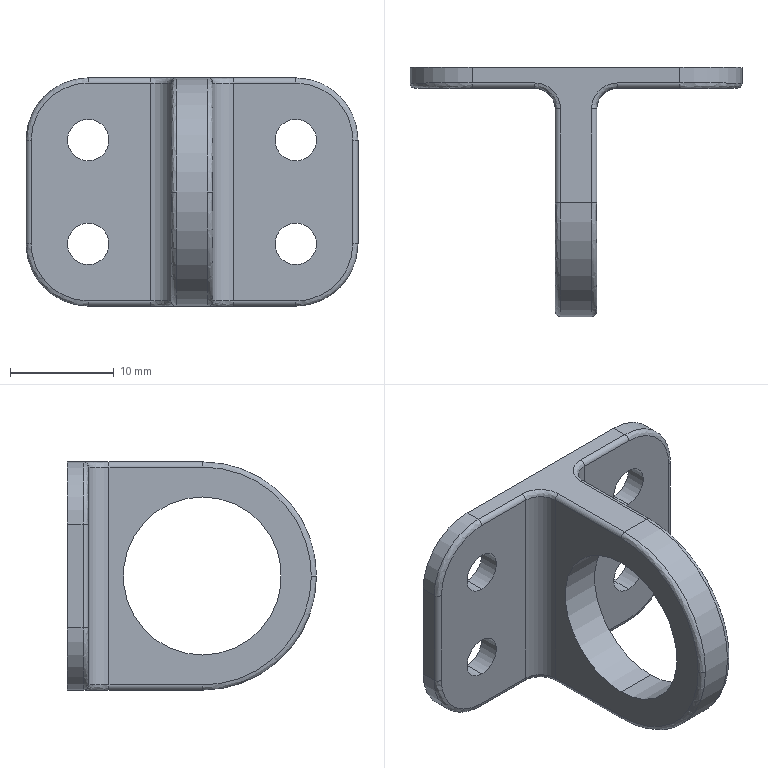Part | SolidWorks | features BaseBody 1 | 1 solid | 48 faces | box 32 x 24 x 22 mm | volume 2271 mm3 | cylinder 27 | spline 12 | plane 9 | commonest cylinder face diameters 1 x10 4 x10 12 x4 15.24 x2 22 x1